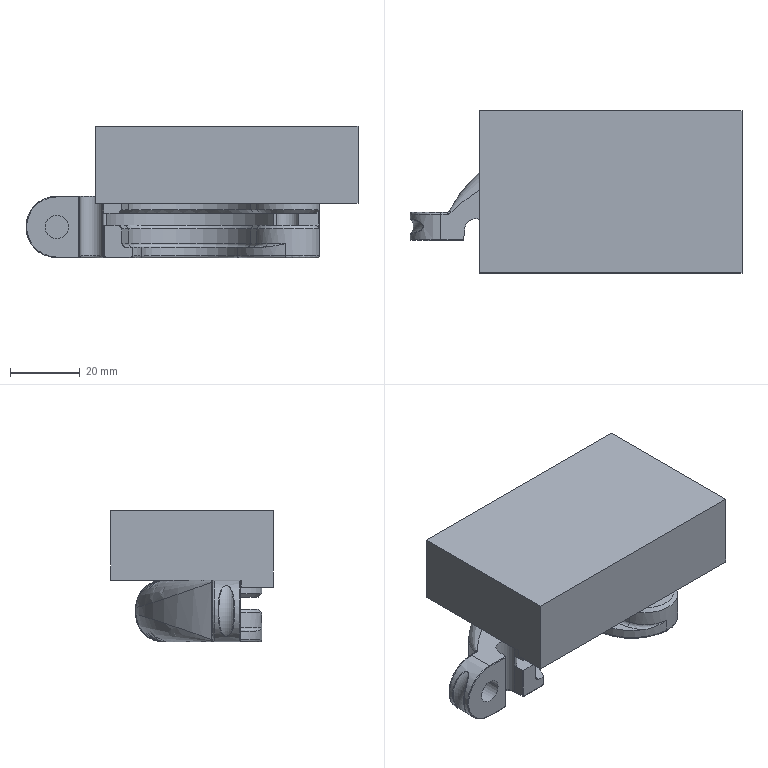NC program | NX | posted with a generic post | part box 94.951 x 46.35 x 37.6 mm
Lines 2348 to 3769 of 15115:
(PLANAR_MILL_3 , TOOL : D16)
N4592 T19 M6
N4594 G54
N4596 G17 G0 G90 X9.895 Y92.003 S5500 M3
N4598 G43 Z50. H19
N4600 Z16.9
N4602 G94 G1 X9.9 Y66.003 F2500.
N4604 Y64.053
N4606 G2 X9.855 Y62.913 R14.4
N4608 X5.16 Y52.857 R15.844
N4610 G3 X2.727 Y50.028 R35.618
N4612 X0.485 Y46.758 R34.794
N4614 X-2.476 Y40.54 R34.63
N4616 X-4.192 Y33.77 R36.295
N4618 X-4.497 Y30.926 R31.475
N4620 X-4.59 Y27.683 R50.37
N4622 X-4.539 Y22.92 R321.072
N4624 X-4.335 Y18.88 R62.671
N4626 X-3.595 Y14.096 R34.207
N4628 X-2.365 Y10.517 R17.742
N4630 X0.004 Y6.991 R13.901
N4632 X2.448 Y5.203 R7.84
N4634 G1 X26.001 Y-5.808
N4636 G0 Z22.4
N4638 X1.495 Y92.001
N4640 Z16.9
N4642 G1 X1.5 Y66.001
N4644 Y64.051
N4646 G2 X1.482 Y63.576 R6.
N4648 X-0.798 Y58.78 R7.444
N4650 G3 X-3.92 Y55.165 R44.018
N4652 X-6.702 Y51.105 R43.194
N4654 X-10.381 Y43.378 R43.03
N4656 X-12.496 Y35.042 R44.695
N4658 X-12.881 Y31.438 R39.875
N4660 X-12.99 Y27.655 R58.77
N4662 X-12.938 Y22.767 R329.472
N4664 X-12.707 Y18.186 R71.071
N4666 X-11.785 Y12.228 R42.607
N4668 X-9.971 Y6.954 R26.142
N4670 X-6.171 Y1.296 R22.301
N4672 X-1.11 Y-2.406 R16.24
N4674 G1 X22.443 Y-13.418
N4676 G0 Z22.4
N4678 X9.895 Y92.003
N4680 Z16.4
N4682 G1 X9.9 Y66.003
N4684 Y64.053
N4686 G2 X9.855 Y62.913 R14.4
N4688 X5.16 Y52.857 R15.844
N4690 G3 X2.727 Y50.028 R35.618
N4692 X0.485 Y46.758 R34.794
N4694 X-2.476 Y40.54 R34.63
N4696 X-4.192 Y33.77 R36.295
N4698 X-4.497 Y30.926 R31.475
N4700 X-4.59 Y27.683 R50.37
N4702 X-4.539 Y22.92 R321.072
N4704 X-4.335 Y18.88 R62.671
N4706 X-3.595 Y14.096 R34.207
N4708 X-2.365 Y10.517 R17.742
N4710 X0.004 Y6.991 R13.901
N4712 X2.448 Y5.203 R7.84
N4714 G1 X26.001 Y-5.808
N4716 G0 Z22.4
N4718 X1.495 Y92.001
N4720 Z16.4
N4722 G1 X1.5 Y66.001
N4724 Y64.051
N4726 G2 X1.482 Y63.576 R6.
N4728 X-0.798 Y58.78 R7.444
N4730 G3 X-3.92 Y55.165 R44.018
N4732 X-6.702 Y51.105 R43.194
N4734 X-10.381 Y43.378 R43.03
N4736 X-12.496 Y35.042 R44.695
N4738 X-12.881 Y31.438 R39.875
N4740 X-12.99 Y27.655 R58.77
N4742 X-12.938 Y22.767 R329.472
N4744 X-12.707 Y18.186 R71.071
N4746 X-11.785 Y12.228 R42.607
N4748 X-9.971 Y6.954 R26.142
N4750 X-6.171 Y1.296 R22.301
N4752 X-1.11 Y-2.406 R16.24
N4754 G1 X22.443 Y-13.418
N4756 G0 Z22.4
N4758 X9.895 Y92.003
N4760 Z15.9
N4762 G1 X9.9 Y66.003
N4764 Y64.053
N4766 G2 X9.855 Y62.913 R14.4
N4768 X5.16 Y52.857 R15.844
N4770 G3 X2.727 Y50.028 R35.618
N4772 X0.485 Y46.758 R34.794
N4774 X-2.476 Y40.54 R34.63
N4776 X-4.192 Y33.77 R36.295
N4778 X-4.497 Y30.926 R31.475
N4780 X-4.59 Y27.683 R50.37
N4782 X-4.539 Y22.92 R321.072
N4784 X-4.335 Y18.88 R62.671
N4786 X-3.595 Y14.096 R34.207
N4788 X-2.365 Y10.517 R17.742
N4790 X0.004 Y6.991 R13.901
N4792 X2.448 Y5.203 R7.84
N4794 G1 X26.001 Y-5.808
N4796 G0 Z22.4
N4798 X1.495 Y92.001
N4800 Z15.9
N4802 G1 X1.5 Y66.001
N4804 Y64.051
N4806 G2 X1.482 Y63.576 R6.
N4808 X-0.798 Y58.78 R7.444
N4810 G3 X-3.92 Y55.165 R44.018
N4812 X-6.702 Y51.105 R43.194
N4814 X-10.381 Y43.378 R43.03
N4816 X-12.496 Y35.042 R44.695
N4818 X-12.881 Y31.438 R39.875
N4820 X-12.99 Y27.655 R58.77
N4822 X-12.938 Y22.767 R329.472
N4824 X-12.707 Y18.186 R71.071
N4826 X-11.785 Y12.228 R42.607
N4828 X-9.971 Y6.954 R26.142
N4830 X-6.171 Y1.296 R22.301
N4832 X-1.11 Y-2.406 R16.24
N4834 G1 X22.443 Y-13.418
N4836 G0 Z22.4
N4838 X9.895 Y92.003
N4840 Z15.4
N4842 G1 X9.9 Y66.003
N4844 Y64.053
N4846 G2 X9.855 Y62.913 R14.4
N4848 X5.16 Y52.857 R15.844
N4850 G3 X2.727 Y50.028 R35.618
N4852 X0.485 Y46.758 R34.794
N4854 X-2.476 Y40.54 R34.63
N4856 X-4.192 Y33.77 R36.295
N4858 X-4.497 Y30.926 R31.475
N4860 X-4.59 Y27.683 R50.37
N4862 X-4.539 Y22.92 R321.072
N4864 X-4.335 Y18.88 R62.671
N4866 X-3.595 Y14.096 R34.207
N4868 X-2.365 Y10.517 R17.742
N4870 X0.004 Y6.991 R13.901
N4872 X2.448 Y5.203 R7.84
N4874 G1 X26.001 Y-5.808
N4876 G0 Z22.4
N4878 X1.495 Y92.001
N4880 Z15.4
N4882 G1 X1.5 Y66.001
N4884 Y64.051
N4886 G2 X1.482 Y63.576 R6.
N4888 X-0.798 Y58.78 R7.444
N4890 G3 X-3.92 Y55.165 R44.018
N4892 X-6.702 Y51.105 R43.194
N4894 X-10.381 Y43.378 R43.03
N4896 X-12.496 Y35.042 R44.695
N4898 X-12.881 Y31.438 R39.875
N4900 X-12.99 Y27.655 R58.77
N4902 X-12.938 Y22.767 R329.472
N4904 X-12.707 Y18.186 R71.071
N4906 X-11.785 Y12.228 R42.607
N4908 X-9.971 Y6.954 R26.142
N4910 X-6.171 Y1.296 R22.301
N4912 X-1.11 Y-2.406 R16.24
N4914 G1 X22.443 Y-13.418
N4916 G0 Z22.4
N4918 X9.895 Y92.003
N4920 Z14.9
N4922 G1 X9.9 Y66.003
N4924 Y64.053
N4926 G2 X9.855 Y62.913 R14.4
N4928 X5.16 Y52.857 R15.844
N4930 G3 X2.727 Y50.028 R35.618
N4932 X0.485 Y46.758 R34.794
N4934 X-2.476 Y40.54 R34.63
N4936 X-4.192 Y33.77 R36.295
N4938 X-4.497 Y30.926 R31.475
N4940 X-4.59 Y27.683 R50.37
N4942 X-4.539 Y22.92 R321.072
N4944 X-4.335 Y18.88 R62.671
N4946 X-3.595 Y14.096 R34.207
N4948 X-2.365 Y10.517 R17.742
N4950 X0.004 Y6.991 R13.901
N4952 X2.448 Y5.203 R7.84
N4954 G1 X26.001 Y-5.808
N4956 G0 Z22.4
N4958 X1.495 Y92.001
N4960 Z14.9
N4962 G1 X1.5 Y66.001
N4964 Y64.051
N4966 G2 X1.482 Y63.576 R6.
N4968 X-0.798 Y58.78 R7.444
N4970 G3 X-3.92 Y55.165 R44.018
N4972 X-6.702 Y51.105 R43.194
N4974 X-10.381 Y43.378 R43.03
N4976 X-12.496 Y35.042 R44.695
N4978 X-12.881 Y31.438 R39.875
N4980 X-12.99 Y27.655 R58.77
N4982 X-12.938 Y22.767 R329.472
N4984 X-12.707 Y18.186 R71.071
N4986 X-11.785 Y12.228 R42.607
N4988 X-9.971 Y6.954 R26.142
N4990 X-6.171 Y1.296 R22.301
N4992 X-1.11 Y-2.406 R16.24
N4994 G1 X22.443 Y-13.418
N4996 G0 Z22.4
N4998 X9.895 Y92.003
N5000 Z14.4
N5002 G1 X9.9 Y66.003
N5004 Y64.053
N5006 G2 X9.855 Y62.913 R14.4
N5008 X5.16 Y52.857 R15.844
N5010 G3 X2.727 Y50.028 R35.618
N5012 X0.485 Y46.758 R34.794
N5014 X-2.476 Y40.54 R34.63
N5016 X-4.192 Y33.77 R36.295
N5018 X-4.497 Y30.926 R31.475
N5020 X-4.59 Y27.683 R50.37
N5022 X-4.539 Y22.92 R321.072
N5024 X-4.335 Y18.88 R62.671
N5026 X-3.595 Y14.096 R34.207
N5028 X-2.365 Y10.517 R17.742
N5030 X0.004 Y6.991 R13.901
N5032 X2.448 Y5.203 R7.84
N5034 G1 X26.001 Y-5.808
N5036 G0 Z22.4
N5038 X1.495 Y92.001
N5040 Z14.4
N5042 G1 X1.5 Y66.001
N5044 Y64.051
N5046 G2 X1.482 Y63.576 R6.
N5048 X-0.798 Y58.78 R7.444
N5050 G3 X-3.92 Y55.165 R44.018
N5052 X-6.702 Y51.105 R43.194
N5054 X-10.381 Y43.378 R43.03
N5056 X-12.496 Y35.042 R44.695
N5058 X-12.881 Y31.438 R39.875
N5060 X-12.99 Y27.655 R58.77
N5062 X-12.938 Y22.767 R329.472
N5064 X-12.707 Y18.186 R71.071
N5066 X-11.785 Y12.228 R42.607
N5068 X-9.971 Y6.954 R26.142
N5070 X-6.171 Y1.296 R22.301
N5072 X-1.11 Y-2.406 R16.24
N5074 G1 X22.443 Y-13.418
N5076 G0 Z22.4
N5078 X9.895 Y92.003
N5080 Z13.9
N5082 G1 X9.9 Y66.003
N5084 Y64.053
N5086 G2 X9.855 Y62.913 R14.4
N5088 X5.16 Y52.857 R15.844
N5090 G3 X2.727 Y50.028 R35.618
N5092 X0.485 Y46.758 R34.794
N5094 X-2.476 Y40.54 R34.63
N5096 X-4.192 Y33.77 R36.295
N5098 X-4.497 Y30.926 R31.475
N5100 X-4.59 Y27.683 R50.37
N5102 X-4.539 Y22.92 R321.072
N5104 X-4.335 Y18.88 R62.671
N5106 X-3.595 Y14.096 R34.207
N5108 X-2.365 Y10.517 R17.742
N5110 X0.004 Y6.991 R13.901
N5112 X2.448 Y5.203 R7.84
N5114 G1 X26.001 Y-5.808
N5116 G0 Z22.4
N5118 X1.495 Y92.001
N5120 Z13.9
N5122 G1 X1.5 Y66.001
N5124 Y64.051
N5126 G2 X1.482 Y63.576 R6.
N5128 X-0.798 Y58.78 R7.444
N5130 G3 X-3.92 Y55.165 R44.018
N5132 X-6.702 Y51.105 R43.194
N5134 X-10.381 Y43.378 R43.03
N5136 X-12.496 Y35.042 R44.695
N5138 X-12.881 Y31.438 R39.875
N5140 X-12.99 Y27.655 R58.77
N5142 X-12.938 Y22.767 R329.472
N5144 X-12.707 Y18.186 R71.071
N5146 X-11.785 Y12.228 R42.607
N5148 X-9.971 Y6.954 R26.142
N5150 X-6.171 Y1.296 R22.301
N5152 X-1.11 Y-2.406 R16.24
N5154 G1 X22.443 Y-13.418
N5156 G0 Z22.4
N5158 X9.895 Y92.003
N5160 Z13.4
N5162 G1 X9.9 Y66.003
N5164 Y64.053
N5166 G2 X9.855 Y62.913 R14.4
N5168 X5.16 Y52.857 R15.844
N5170 G3 X2.727 Y50.028 R35.618
N5172 X0.485 Y46.758 R34.794
N5174 X-2.476 Y40.54 R34.63
N5176 X-4.192 Y33.77 R36.295
N5178 X-4.497 Y30.926 R31.475
N5180 X-4.59 Y27.683 R50.37
N5182 X-4.539 Y22.92 R321.072
N5184 X-4.335 Y18.88 R62.671
N5186 X-3.595 Y14.096 R34.207
N5188 X-2.365 Y10.517 R17.742
N5190 X0.004 Y6.991 R13.901
N5192 X2.448 Y5.203 R7.84
N5194 G1 X26.001 Y-5.808
N5196 G0 Z22.4
N5198 X1.495 Y92.001
N5200 Z13.4
N5202 G1 X1.5 Y66.001
N5204 Y64.051
N5206 G2 X1.482 Y63.576 R6.
N5208 X-0.798 Y58.78 R7.444
N5210 G3 X-3.92 Y55.165 R44.018
N5212 X-6.702 Y51.105 R43.194
N5214 X-10.381 Y43.378 R43.03
N5216 X-12.496 Y35.042 R44.695
N5218 X-12.881 Y31.438 R39.875
N5220 X-12.99 Y27.655 R58.77
N5222 X-12.938 Y22.767 R329.472
N5224 X-12.707 Y18.186 R71.071
N5226 X-11.785 Y12.228 R42.607
N5228 X-9.971 Y6.954 R26.142
N5230 X-6.171 Y1.296 R22.301
N5232 X-1.11 Y-2.406 R16.24
N5234 G1 X22.443 Y-13.418
N5236 G0 Z22.4
N5238 X9.895 Y92.003
N5240 Z12.9
N5242 G1 X9.9 Y66.003
N5244 Y64.053
N5246 G2 X9.855 Y62.913 R14.4
N5248 X5.16 Y52.857 R15.844
N5250 G3 X2.727 Y50.028 R35.618
N5252 X0.485 Y46.758 R34.794
N5254 X-2.476 Y40.54 R34.63
N5256 X-4.192 Y33.77 R36.295
N5258 X-4.497 Y30.926 R31.475
N5260 X-4.59 Y27.683 R50.37
N5262 X-4.539 Y22.92 R321.072
N5264 X-4.335 Y18.88 R62.671
N5266 X-3.595 Y14.096 R34.207
N5268 X-2.365 Y10.517 R17.742
N5270 X0.004 Y6.991 R13.901
N5272 X2.448 Y5.203 R7.84
N5274 G1 X26.001 Y-5.808
N5276 G0 Z22.4
N5278 X1.495 Y92.001
N5280 Z12.9
N5282 G1 X1.5 Y66.001
N5284 Y64.051
N5286 G2 X1.482 Y63.576 R6.
N5288 X-0.798 Y58.78 R7.444
N5290 G3 X-3.92 Y55.165 R44.018
N5292 X-6.702 Y51.105 R43.194
N5294 X-10.381 Y43.378 R43.03
N5296 X-12.496 Y35.042 R44.695
N5298 X-12.881 Y31.438 R39.875
N5300 X-12.99 Y27.655 R58.77
N5302 X-12.938 Y22.767 R329.472
N5304 X-12.707 Y18.186 R71.071
N5306 X-11.785 Y12.228 R42.607
N5308 X-9.971 Y6.954 R26.142
N5310 X-6.171 Y1.296 R22.301
N5312 X-1.11 Y-2.406 R16.24
N5314 G1 X22.443 Y-13.418
N5316 G0 Z22.4
N5318 X9.895 Y92.003
N5320 Z12.4
N5322 G1 X9.9 Y66.003
N5324 Y64.053
N5326 G2 X9.855 Y62.913 R14.4
N5328 X5.16 Y52.857 R15.844
N5330 G3 X2.727 Y50.028 R35.618
N5332 X0.485 Y46.758 R34.794
N5334 X-2.476 Y40.54 R34.63
N5336 X-4.192 Y33.77 R36.295
N5338 X-4.497 Y30.926 R31.475
N5340 X-4.59 Y27.683 R50.37
N5342 X-4.539 Y22.92 R321.072
N5344 X-4.335 Y18.88 R62.671
N5346 X-3.595 Y14.096 R34.207
N5348 X-2.365 Y10.517 R17.742
N5350 X0.004 Y6.991 R13.901
N5352 X2.448 Y5.203 R7.84
N5354 G1 X26.001 Y-5.808
N5356 G0 Z22.4
N5358 X1.495 Y92.001
N5360 Z12.4
N5362 G1 X1.5 Y66.001
N5364 Y64.051
N5366 G2 X1.482 Y63.576 R6.
N5368 X-0.798 Y58.78 R7.444
N5370 G3 X-3.92 Y55.165 R44.018
N5372 X-6.702 Y51.105 R43.194
N5374 X-10.381 Y43.378 R43.03
N5376 X-12.496 Y35.042 R44.695
N5378 X-12.881 Y31.438 R39.875
N5380 X-12.99 Y27.655 R58.77
N5382 X-12.938 Y22.767 R329.472
N5384 X-12.707 Y18.186 R71.071
N5386 X-11.785 Y12.228 R42.607
N5388 X-9.971 Y6.954 R26.142
N5390 X-6.171 Y1.296 R22.301
N5392 X-1.11 Y-2.406 R16.24
N5394 G1 X22.443 Y-13.418
N5396 G0 Z22.4
N5398 X9.895 Y92.003
N5400 Z11.9
N5402 G1 X9.9 Y66.003
N5404 Y64.053
N5406 G2 X9.855 Y62.913 R14.4
N5408 X5.16 Y52.857 R15.844
N5410 G3 X2.727 Y50.028 R35.618
N5412 X0.485 Y46.758 R34.794
N5414 X-2.476 Y40.54 R34.63
N5416 X-4.192 Y33.77 R36.295
N5418 X-4.497 Y30.926 R31.475
N5420 X-4.59 Y27.683 R50.37
N5422 X-4.539 Y22.92 R321.072
N5424 X-4.335 Y18.88 R62.671
N5426 X-3.595 Y14.096 R34.207
N5428 X-2.365 Y10.517 R17.742
N5430 X0.004 Y6.991 R13.901
N5432 X2.448 Y5.203 R7.84
N5434 G1 X26.001 Y-5.808
N5436 G0 Z22.4
N5438 X1.495 Y92.001
N5440 Z11.9
N5442 G1 X1.5 Y66.001
N5444 Y64.051
N5446 G2 X1.482 Y63.576 R6.
N5448 X-0.798 Y58.78 R7.444
N5450 G3 X-3.92 Y55.165 R44.018
N5452 X-6.702 Y51.105 R43.194
N5454 X-10.381 Y43.378 R43.03
N5456 X-12.496 Y35.042 R44.695
N5458 X-12.881 Y31.438 R39.875
N5460 X-12.99 Y27.655 R58.77
N5462 X-12.938 Y22.767 R329.472
N5464 X-12.707 Y18.186 R71.071
N5466 X-11.785 Y12.228 R42.607
N5468 X-9.971 Y6.954 R26.142
N5470 X-6.171 Y1.296 R22.301
N5472 X-1.11 Y-2.406 R16.24
N5474 G1 X22.443 Y-13.418
N5476 G0 Z22.4
N5478 X9.895 Y92.003
N5480 Z11.4
N5482 G1 X9.9 Y66.003
N5484 Y64.053
N5486 G2 X9.855 Y62.913 R14.4
N5488 X5.16 Y52.857 R15.844
N5490 G3 X2.727 Y50.028 R35.618
N5492 X0.485 Y46.758 R34.794
N5494 X-2.476 Y40.54 R34.63
N5496 X-4.192 Y33.77 R36.295
N5498 X-4.497 Y30.926 R31.475
N5500 X-4.59 Y27.683 R50.37
N5502 X-4.539 Y22.92 R321.072
N5504 X-4.335 Y18.88 R62.671
N5506 X-3.595 Y14.096 R34.207
N5508 X-2.365 Y10.517 R17.742
N5510 X0.004 Y6.991 R13.901
N5512 X2.448 Y5.203 R7.84
N5514 G1 X26.001 Y-5.808
N5516 G0 Z22.4
N5518 X1.495 Y92.001
N5520 Z11.4
N5522 G1 X1.5 Y66.001
N5524 Y64.051
N5526 G2 X1.482 Y63.576 R6.
N5528 X-0.798 Y58.78 R7.444
N5530 G3 X-3.92 Y55.165 R44.018
N5532 X-6.702 Y51.105 R43.194
N5534 X-10.381 Y43.378 R43.03
N5536 X-12.496 Y35.042 R44.695
N5538 X-12.881 Y31.438 R39.875
N5540 X-12.99 Y27.655 R58.77
N5542 X-12.938 Y22.767 R329.472
N5544 X-12.707 Y18.186 R71.071
N5546 X-11.785 Y12.228 R42.607
N5548 X-9.971 Y6.954 R26.142
N5550 X-6.171 Y1.296 R22.301
N5552 X-1.11 Y-2.406 R16.24
N5554 G1 X22.443 Y-13.418
N5556 G0 Z22.4
N5558 X9.895 Y92.003
N5560 Z10.9
N5562 G1 X9.9 Y66.003
N5564 Y64.053
N5566 G2 X9.855 Y62.913 R14.4
N5568 X5.16 Y52.857 R15.844
N5570 G3 X2.727 Y50.028 R35.618
N5572 X0.485 Y46.758 R34.794
N5574 X-2.476 Y40.54 R34.63
N5576 X-4.192 Y33.77 R36.295
N5578 X-4.497 Y30.926 R31.475
N5580 X-4.59 Y27.683 R50.37
N5582 X-4.539 Y22.92 R321.072
N5584 X-4.335 Y18.88 R62.671
N5586 X-3.595 Y14.096 R34.207
N5588 X-2.365 Y10.517 R17.742
N5590 X0.004 Y6.991 R13.901
N5592 X2.448 Y5.203 R7.84
N5594 G1 X26.001 Y-5.808
N5596 G0 Z22.4
N5598 X1.495 Y92.001
N5600 Z10.9
N5602 G1 X1.5 Y66.001
N5604 Y64.051
N5606 G2 X1.482 Y63.576 R6.
N5608 X-0.798 Y58.78 R7.444
N5610 G3 X-3.92 Y55.165 R44.018
N5612 X-6.702 Y51.105 R43.194
N5614 X-10.381 Y43.378 R43.03
N5616 X-12.496 Y35.042 R44.695
N5618 X-12.881 Y31.438 R39.875
N5620 X-12.99 Y27.655 R58.77
N5622 X-12.938 Y22.767 R329.472
N5624 X-12.707 Y18.186 R71.071
N5626 X-11.785 Y12.228 R42.607
N5628 X-9.971 Y6.954 R26.142
N5630 X-6.171 Y1.296 R22.301
N5632 X-1.11 Y-2.406 R16.24
N5634 G1 X22.443 Y-13.418
N5636 G0 Z22.4
N5638 X9.895 Y92.003
N5640 Z10.4
N5642 G1 X9.9 Y66.003
N5644 Y64.053
N5646 G2 X9.855 Y62.913 R14.4
N5648 X5.16 Y52.857 R15.844
N5650 G3 X2.727 Y50.028 R35.618
N5652 X0.485 Y46.758 R34.794
N5654 X-2.476 Y40.54 R34.63
N5656 X-4.192 Y33.77 R36.295
N5658 X-4.497 Y30.926 R31.475
N5660 X-4.59 Y27.683 R50.37
N5662 X-4.539 Y22.92 R321.072
N5664 X-4.335 Y18.88 R62.671
N5666 X-3.595 Y14.096 R34.207
N5668 X-2.365 Y10.517 R17.742
N5670 X0.004 Y6.991 R13.901
N5672 X2.448 Y5.203 R7.84
N5674 G1 X26.001 Y-5.808
N5676 G0 Z22.4
N5678 X1.495 Y92.001
N5680 Z10.4
N5682 G1 X1.5 Y66.001
N5684 Y64.051
N5686 G2 X1.482 Y63.576 R6.
N5688 X-0.798 Y58.78 R7.444
N5690 G3 X-3.92 Y55.165 R44.018
N5692 X-6.702 Y51.105 R43.194
N5694 X-10.381 Y43.378 R43.03
N5696 X-12.496 Y35.042 R44.695
N5698 X-12.881 Y31.438 R39.875
N5700 X-12.99 Y27.655 R58.77
N5702 X-12.938 Y22.767 R329.472
N5704 X-12.707 Y18.186 R71.071
N5706 X-11.785 Y12.228 R42.607
N5708 X-9.971 Y6.954 R26.142
N5710 X-6.171 Y1.296 R22.301
N5712 X-1.11 Y-2.406 R16.24
N5714 G1 X22.443 Y-13.418
N5716 G0 Z22.4
N5718 X9.895 Y92.003
N5720 Z9.9
N5722 G1 X9.9 Y66.003
N5724 Y64.053
N5726 G2 X9.855 Y62.913 R14.4
N5728 X5.16 Y52.857 R15.844
N5730 G3 X2.727 Y50.028 R35.618
N5732 X0.485 Y46.758 R34.794
N5734 X-2.476 Y40.54 R34.63
N5736 X-4.192 Y33.77 R36.295
N5738 X-4.497 Y30.926 R31.475
N5740 X-4.59 Y27.683 R50.37
N5742 X-4.539 Y22.92 R321.072
N5744 X-4.335 Y18.88 R62.671
N5746 X-3.595 Y14.096 R34.207
N5748 X-2.365 Y10.517 R17.742
N5750 X0.004 Y6.991 R13.901
N5752 X2.448 Y5.203 R7.84
N5754 G1 X26.001 Y-5.808
N5756 G0 Z22.4
N5758 X1.495 Y92.001
N5760 Z9.9
N5762 G1 X1.5 Y66.001
N5764 Y64.051
N5766 G2 X1.482 Y63.576 R6.
N5768 X-0.798 Y58.78 R7.444
N5770 G3 X-3.92 Y55.165 R44.018
N5772 X-6.702 Y51.105 R43.194
N5774 X-10.381 Y43.378 R43.03
N5776 X-12.496 Y35.042 R44.695
N5778 X-12.881 Y31.438 R39.875
N5780 X-12.99 Y27.655 R58.77
N5782 X-12.938 Y22.767 R329.472
N5784 X-12.707 Y18.186 R71.071
N5786 X-11.785 Y12.228 R42.607
N5788 X-9.971 Y6.954 R26.142
N5790 X-6.171 Y1.296 R22.301
N5792 X-1.11 Y-2.406 R16.24
N5794 G1 X22.443 Y-13.418
N5796 G0 Z22.4
N5798 X9.895 Y92.003
N5800 Z9.4
N5802 G1 X9.9 Y66.003
N5804 Y64.053
N5806 G2 X9.855 Y62.913 R14.4
N5808 X5.16 Y52.857 R15.844
N5810 G3 X2.727 Y50.028 R35.618
N5812 X0.485 Y46.758 R34.794
N5814 X-2.476 Y40.54 R34.63
N5816 X-4.192 Y33.77 R36.295
N5818 X-4.497 Y30.926 R31.475
N5820 X-4.59 Y27.683 R50.37
N5822 X-4.539 Y22.92 R321.072
N5824 X-4.335 Y18.88 R62.671
N5826 X-3.595 Y14.096 R34.207
N5828 X-2.365 Y10.517 R17.742
N5830 X0.004 Y6.991 R13.901
N5832 X2.448 Y5.203 R7.84
N5834 G1 X26.001 Y-5.808
N5836 G0 Z22.4
N5838 X1.495 Y92.001
N5840 Z9.4
N5842 G1 X1.5 Y66.001
N5844 Y64.051
N5846 G2 X1.482 Y63.576 R6.
N5848 X-0.798 Y58.78 R7.444
N5850 G3 X-3.92 Y55.165 R44.018
N5852 X-6.702 Y51.105 R43.194
N5854 X-10.381 Y43.378 R43.03
N5856 X-12.496 Y35.042 R44.695
N5858 X-12.881 Y31.438 R39.875
N5860 X-12.99 Y27.655 R58.77
N5862 X-12.938 Y22.767 R329.472
N5864 X-12.707 Y18.186 R71.071
N5866 X-11.785 Y12.228 R42.607
N5868 X-9.971 Y6.954 R26.142
N5870 X-6.171 Y1.296 R22.301
N5872 X-1.11 Y-2.406 R16.24
N5874 G1 X22.443 Y-13.418
N5876 G0 Z22.4
N5878 X9.895 Y92.003
N5880 Z8.9
N5882 G1 X9.9 Y66.003
N5884 Y64.053
N5886 G2 X9.855 Y62.913 R14.4
N5888 X5.16 Y52.857 R15.844
N5890 G3 X2.727 Y50.028 R35.618
N5892 X0.485 Y46.758 R34.794
N5894 X-2.476 Y40.54 R34.63
N5896 X-4.192 Y33.77 R36.295
N5898 X-4.497 Y30.926 R31.475
N5900 X-4.59 Y27.683 R50.37
N5902 X-4.539 Y22.92 R321.072
N5904 X-4.335 Y18.88 R62.671
N5906 X-3.595 Y14.096 R34.207
N5908 X-2.365 Y10.517 R17.742
N5910 X0.004 Y6.991 R13.901
N5912 X2.448 Y5.203 R7.84
N5914 G1 X26.001 Y-5.808
N5916 G0 Z22.4
N5918 X1.495 Y92.001
N5920 Z8.9
N5922 G1 X1.5 Y66.001
N5924 Y64.051
N5926 G2 X1.482 Y63.576 R6.
N5928 X-0.798 Y58.78 R7.444
N5930 G3 X-3.92 Y55.165 R44.018
N5932 X-6.702 Y51.105 R43.194
N5934 X-10.381 Y43.378 R43.03
N5936 X-12.496 Y35.042 R44.695
N5938 X-12.881 Y31.438 R39.875
N5940 X-12.99 Y27.655 R58.77
N5942 X-12.938 Y22.767 R329.472
N5944 X-12.707 Y18.186 R71.071
N5946 X-11.785 Y12.228 R42.607
N5948 X-9.971 Y6.954 R26.142
N5950 X-6.171 Y1.296 R22.301
N5952 X-1.11 Y-2.406 R16.24
N5954 G1 X22.443 Y-13.418
N5956 G0 Z22.4
N5958 X9.895 Y92.003
N5960 Z8.4
N5962 G1 X9.9 Y66.003
N5964 Y64.053
N5966 G2 X9.855 Y62.913 R14.4
N5968 X5.16 Y52.857 R15.844
N5970 G3 X2.727 Y50.028 R35.618
N5972 X0.485 Y46.758 R34.794
N5974 X-2.476 Y40.54 R34.63
N5976 X-4.192 Y33.77 R36.295
N5978 X-4.497 Y30.926 R31.475
N5980 X-4.59 Y27.683 R50.37
N5982 X-4.539 Y22.92 R321.072
N5984 X-4.335 Y18.88 R62.671
N5986 X-3.595 Y14.096 R34.207
N5988 X-2.365 Y10.517 R17.742
N5990 X0.004 Y6.991 R13.901
N5992 X2.448 Y5.203 R7.84
N5994 G1 X26.001 Y-5.808
N5996 G0 Z22.4
N5998 X1.495 Y92.001
N6000 Z8.4
N6002 G1 X1.5 Y66.001
N6004 Y64.051
N6006 G2 X1.482 Y63.576 R6.
N6008 X-0.798 Y58.78 R7.444
N6010 G3 X-3.92 Y55.165 R44.018
N6012 X-6.702 Y51.105 R43.194
N6014 X-10.381 Y43.378 R43.03
N6016 X-12.496 Y35.042 R44.695
N6018 X-12.881 Y31.438 R39.875
N6020 X-12.99 Y27.655 R58.77
N6022 X-12.938 Y22.767 R329.472
N6024 X-12.707 Y18.186 R71.071
N6026 X-11.785 Y12.228 R42.607
N6028 X-9.971 Y6.954 R26.142
N6030 X-6.171 Y1.296 R22.301
N6032 X-1.11 Y-2.406 R16.24
N6034 G1 X22.443 Y-13.418
N6036 G0 Z22.4
N6038 X9.895 Y92.003
N6040 Z7.9
N6042 G1 X9.9 Y66.003
N6044 Y64.053
N6046 G2 X9.855 Y62.913 R14.4
N6048 X5.16 Y52.857 R15.844
N6050 G3 X2.727 Y50.028 R35.618
N6052 X0.485 Y46.758 R34.794
N6054 X-2.476 Y40.54 R34.63
N6056 X-4.192 Y33.77 R36.295
N6058 X-4.497 Y30.926 R31.475
N6060 X-4.59 Y27.683 R50.37
N6062 X-4.539 Y22.92 R321.072
N6064 X-4.335 Y18.88 R62.671
N6066 X-3.595 Y14.096 R34.207
N6068 X-2.365 Y10.517 R17.742
N6070 X0.004 Y6.991 R13.901
N6072 X2.448 Y5.203 R7.84
N6074 G1 X26.001 Y-5.808
N6076 G0 Z22.4
N6078 X1.495 Y92.001
N6080 Z7.9
N6082 G1 X1.5 Y66.001
N6084 Y64.051
N6086 G2 X1.482 Y63.576 R6.
N6088 X-0.798 Y58.78 R7.444
N6090 G3 X-3.92 Y55.165 R44.018
N6092 X-6.702 Y51.105 R43.194
N6094 X-10.381 Y43.378 R43.03
N6096 X-12.496 Y35.042 R44.695
N6098 X-12.881 Y31.438 R39.875
N6100 X-12.99 Y27.655 R58.77
N6102 X-12.938 Y22.767 R329.472
N6104 X-12.707 Y18.186 R71.071
N6106 X-11.785 Y12.228 R42.607
N6108 X-9.971 Y6.954 R26.142
N6110 X-6.171 Y1.296 R22.301
N6112 X-1.11 Y-2.406 R16.24
N6114 G1 X22.443 Y-13.418
N6116 G0 Z22.4
N6118 X9.895 Y92.003
N6120 Z7.4
N6122 G1 X9.9 Y66.003
N6124 Y64.053
N6126 G2 X9.855 Y62.913 R14.4
N6128 X5.16 Y52.857 R15.844
N6130 G3 X2.727 Y50.028 R35.618
N6132 X0.485 Y46.758 R34.794
N6134 X-2.476 Y40.54 R34.63
N6136 X-4.192 Y33.77 R36.295
N6138 X-4.497 Y30.926 R31.475
N6140 X-4.59 Y27.683 R50.37
N6142 X-4.539 Y22.92 R321.072
N6144 X-4.335 Y18.88 R62.671
N6146 X-3.595 Y14.096 R34.207
N6148 X-2.365 Y10.517 R17.742
N6150 X0.004 Y6.991 R13.901
N6152 X2.448 Y5.203 R7.84
N6154 G1 X26.001 Y-5.808
N6156 G0 Z22.4
N6158 X1.495 Y92.001
N6160 Z7.4
N6162 G1 X1.5 Y66.001
N6164 Y64.051
N6166 G2 X1.482 Y63.576 R6.
N6168 X-0.798 Y58.78 R7.444
N6170 G3 X-3.92 Y55.165 R44.018
N6172 X-6.702 Y51.105 R43.194
N6174 X-10.381 Y43.378 R43.03
N6176 X-12.496 Y35.042 R44.695
N6178 X-12.881 Y31.438 R39.875
N6180 X-12.99 Y27.655 R58.77
N6182 X-12.938 Y22.767 R329.472
N6184 X-12.707 Y18.186 R71.071
N6186 X-11.785 Y12.228 R42.607
N6188 X-9.971 Y6.954 R26.142
N6190 X-6.171 Y1.296 R22.301
N6192 X-1.11 Y-2.406 R16.24
N6194 G1 X22.443 Y-13.418
N6196 G0 Z22.4
N6198 X9.895 Y92.003
N6200 Z6.9
N6202 G1 X9.9 Y66.003
N6204 Y64.053
N6206 G2 X9.855 Y62.913 R14.4
N6208 X5.16 Y52.857 R15.844
N6210 G3 X2.727 Y50.028 R35.618
N6212 X0.485 Y46.758 R34.794
N6214 X-2.476 Y40.54 R34.63
N6216 X-4.192 Y33.77 R36.295
N6218 X-4.497 Y30.926 R31.475
N6220 X-4.59 Y27.683 R50.37
N6222 X-4.539 Y22.92 R321.072
N6224 X-4.335 Y18.88 R62.671
N6226 X-3.595 Y14.096 R34.207
N6228 X-2.365 Y10.517 R17.742
N6230 X0.004 Y6.991 R13.901
N6232 X2.448 Y5.203 R7.84
N6234 G1 X26.001 Y-5.808
N6236 G0 Z22.4
N6238 X1.495 Y92.001
N6240 Z6.9
N6242 G1 X1.5 Y66.001
N6244 Y64.051
N6246 G2 X1.482 Y63.576 R6.
N6248 X-0.798 Y58.78 R7.444
N6250 G3 X-3.92 Y55.165 R44.018
N6252 X-6.702 Y51.105 R43.194
N6254 X-10.381 Y43.378 R43.03
N6256 X-12.496 Y35.042 R44.695
N6258 X-12.881 Y31.438 R39.875
N6260 X-12.99 Y27.655 R58.77
N6262 X-12.938 Y22.767 R329.472
N6264 X-12.707 Y18.186 R71.071
N6266 X-11.785 Y12.228 R42.607
N6268 X-9.971 Y6.954 R26.142
N6270 X-6.171 Y1.296 R22.301
N6272 X-1.11 Y-2.406 R16.24
N6274 G1 X22.443 Y-13.418
N6276 G0 Z22.4
N6278 X9.895 Y92.003
N6280 Z6.4
N6282 G1 X9.9 Y66.003
N6284 Y64.053
N6286 G2 X9.855 Y62.913 R14.4
N6288 X5.16 Y52.857 R15.844
N6290 G3 X2.727 Y50.028 R35.618
N6292 X0.485 Y46.758 R34.794
N6294 X-2.476 Y40.54 R34.63
N6296 X-4.192 Y33.77 R36.295
N6298 X-4.497 Y30.926 R31.475
N6300 X-4.59 Y27.683 R50.37
N6302 X-4.539 Y22.92 R321.072
N6304 X-4.335 Y18.88 R62.671
N6306 X-3.595 Y14.096 R34.207
N6308 X-2.365 Y10.517 R17.742
N6310 X0.004 Y6.991 R13.901
N6312 X2.448 Y5.203 R7.84
N6314 G1 X26.001 Y-5.808
N6316 G0 Z22.4
N6318 X1.495 Y92.001
N6320 Z6.4
N6322 G1 X1.5 Y66.001
N6324 Y64.051
N6326 G2 X1.482 Y63.576 R6.
N6328 X-0.798 Y58.78 R7.444
N6330 G3 X-3.92 Y55.165 R44.018
N6332 X-6.702 Y51.105 R43.194
N6334 X-10.381 Y43.378 R43.03
N6336 X-12.496 Y35.042 R44.695
N6338 X-12.881 Y31.438 R39.875
N6340 X-12.99 Y27.655 R58.77
N6342 X-12.938 Y22.767 R329.472
N6344 X-12.707 Y18.186 R71.071
N6346 X-11.785 Y12.228 R42.607
N6348 X-9.971 Y6.954 R26.142
N6350 X-6.171 Y1.296 R22.301
N6352 X-1.11 Y-2.406 R16.24
N6354 G1 X22.443 Y-13.418
N6356 G0 Z22.4
N6358 X9.895 Y92.003
N6360 Z5.9
N6362 G1 X9.9 Y66.003
N6364 Y64.053
N6366 G2 X9.855 Y62.913 R14.4
N6368 X5.16 Y52.857 R15.844
N6370 G3 X2.727 Y50.028 R35.618
N6372 X0.485 Y46.758 R34.794
N6374 X-2.476 Y40.54 R34.63
N6376 X-4.192 Y33.77 R36.295
N6378 X-4.497 Y30.926 R31.475
N6380 X-4.59 Y27.683 R50.37
N6382 X-4.539 Y22.92 R321.072
N6384 X-4.335 Y18.88 R62.671
N6386 X-3.595 Y14.096 R34.207
N6388 X-2.365 Y10.517 R17.742
N6390 X0.004 Y6.991 R13.901
N6392 X2.448 Y5.203 R7.84
N6394 G1 X26.001 Y-5.808
N6396 G0 Z22.4
N6398 X1.495 Y92.001
N6400 Z5.9
N6402 G1 X1.5 Y66.001
N6404 Y64.051
N6406 G2 X1.482 Y63.576 R6.
N6408 X-0.798 Y58.78 R7.444
N6410 G3 X-3.92 Y55.165 R44.018
N6412 X-6.702 Y51.105 R43.194
N6414 X-10.381 Y43.378 R43.03
N6416 X-12.496 Y35.042 R44.695
N6418 X-12.881 Y31.438 R39.875
N6420 X-12.99 Y27.655 R58.77
N6422 X-12.938 Y22.767 R329.472
N6424 X-12.707 Y18.186 R71.071
N6426 X-11.785 Y12.228 R42.607
N6428 X-9.971 Y6.954 R26.142
N6430 X-6.171 Y1.296 R22.301
N6432 X-1.11 Y-2.406 R16.24
N6434 G1 X22.443 Y-13.418
N6436 G0 Z22.4
N6438 X9.895 Y92.003
N6440 Z5.4
N6442 G1 X9.9 Y66.003
N6444 Y64.053
N6446 G2 X9.855 Y62.913 R14.4
N6448 X5.16 Y52.857 R15.844
N6450 G3 X2.727 Y50.028 R35.618
N6452 X0.485 Y46.758 R34.794
N6454 X-2.476 Y40.54 R34.63
N6456 X-4.192 Y33.77 R36.295
N6458 X-4.497 Y30.926 R31.475
N6460 X-4.59 Y27.683 R50.37
N6462 X-4.539 Y22.92 R321.072
N6464 X-4.335 Y18.88 R62.671
N6466 X-3.595 Y14.096 R34.207
N6468 X-2.365 Y10.517 R17.742
N6470 X0.004 Y6.991 R13.901
N6472 X2.448 Y5.203 R7.84
N6474 G1 X26.001 Y-5.808
N6476 G0 Z22.4
N6478 X1.495 Y92.001
N6480 Z5.4
N6482 G1 X1.5 Y66.001
N6484 Y64.051
N6486 G2 X1.482 Y63.576 R6.
N6488 X-0.798 Y58.78 R7.444
N6490 G3 X-3.92 Y55.165 R44.018
N6492 X-6.702 Y51.105 R43.194
N6494 X-10.381 Y43.378 R43.03
N6496 X-12.496 Y35.042 R44.695
N6498 X-12.881 Y31.438 R39.875
N6500 X-12.99 Y27.655 R58.77
N6502 X-12.938 Y22.767 R329.472
N6504 X-12.707 Y18.186 R71.071
N6506 X-11.785 Y12.228 R42.607
N6508 X-9.971 Y6.954 R26.142
N6510 X-6.171 Y1.296 R22.301
N6512 X-1.11 Y-2.406 R16.24
N6514 G1 X22.443 Y-13.418
N6516 G0 Z22.4
N6518 X9.895 Y92.003
N6520 Z4.9
N6522 G1 X9.9 Y66.003
N6524 Y64.053
N6526 G2 X9.855 Y62.913 R14.4
N6528 X5.16 Y52.857 R15.844
N6530 G3 X2.727 Y50.028 R35.618
N6532 X0.485 Y46.758 R34.794
N6534 X-2.476 Y40.54 R34.63
N6536 X-4.192 Y33.77 R36.295
N6538 X-4.497 Y30.926 R31.475
N6540 X-4.59 Y27.683 R50.37
N6542 X-4.539 Y22.92 R321.072
N6544 X-4.335 Y18.88 R62.671
N6546 X-3.595 Y14.096 R34.207
N6548 X-2.365 Y10.517 R17.742
N6550 X0.004 Y6.991 R13.901
N6552 X2.448 Y5.203 R7.84
N6554 G1 X26.001 Y-5.808
N6556 G0 Z22.4
N6558 X1.495 Y92.001
N6560 Z4.9
N6562 G1 X1.5 Y66.001
N6564 Y64.051
N6566 G2 X1.482 Y63.576 R6.
N6568 X-0.798 Y58.78 R7.444
N6570 G3 X-3.92 Y55.165 R44.018
N6572 X-6.702 Y51.105 R43.194
N6574 X-10.381 Y43.378 R43.03
N6576 X-12.496 Y35.042 R44.695
N6578 X-12.881 Y31.438 R39.875
N6580 X-12.99 Y27.655 R58.77
N6582 X-12.938 Y22.767 R329.472
N6584 X-12.707 Y18.186 R71.071
N6586 X-11.785 Y12.228 R42.607
N6588 X-9.971 Y6.954 R26.142
N6590 X-6.171 Y1.296 R22.301
N6592 X-1.11 Y-2.406 R16.24
N6594 G1 X22.443 Y-13.418
N6596 G0 Z22.4
N6598 X9.895 Y92.003
N6600 Z4.4
N6602 G1 X9.9 Y66.003
N6604 Y64.053
N6606 G2 X9.855 Y62.913 R14.4
N6608 X5.16 Y52.857 R15.844
N6610 G3 X2.727 Y50.028 R35.618
N6612 X0.485 Y46.758 R34.794
N6614 X-2.476 Y40.54 R34.63
N6616 X-4.192 Y33.77 R36.295
N6618 X-4.497 Y30.926 R31.475
N6620 X-4.59 Y27.683 R50.37
N6622 X-4.539 Y22.92 R321.072
N6624 X-4.335 Y18.88 R62.671
N6626 X-3.595 Y14.096 R34.207
N6628 X-2.365 Y10.517 R17.742
N6630 X0.004 Y6.991 R13.901
N6632 X2.448 Y5.203 R7.84
N6634 G1 X26.001 Y-5.808
N6636 G0 Z22.4
N6638 X1.495 Y92.001
N6640 Z4.4
N6642 G1 X1.5 Y66.001
N6644 Y64.051
N6646 G2 X1.482 Y63.576 R6.
N6648 X-0.798 Y58.78 R7.444
N6650 G3 X-3.92 Y55.165 R44.018
N6652 X-6.702 Y51.105 R43.194
N6654 X-10.381 Y43.378 R43.03
N6656 X-12.496 Y35.042 R44.695
N6658 X-12.881 Y31.438 R39.875
N6660 X-12.99 Y27.655 R58.77
N6662 X-12.938 Y22.767 R329.472
N6664 X-12.707 Y18.186 R71.071
N6666 X-11.785 Y12.228 R42.607
N6668 X-9.971 Y6.954 R26.142
N6670 X-6.171 Y1.296 R22.301
N6672 X-1.11 Y-2.406 R16.24
N6674 G1 X22.443 Y-13.418
N6676 G0 Z22.4
N6678 X9.895 Y92.003
N6680 Z3.9
N6682 G1 X9.9 Y66.003
N6684 Y64.053
N6686 G2 X9.855 Y62.913 R14.4
N6688 X5.16 Y52.857 R15.844
N6690 G3 X2.727 Y50.028 R35.618
N6692 X0.485 Y46.758 R34.794
N6694 X-2.476 Y40.54 R34.63
N6696 X-4.192 Y33.77 R36.295
N6698 X-4.497 Y30.926 R31.475
N6700 X-4.59 Y27.683 R50.37
N6702 X-4.539 Y22.92 R321.072
N6704 X-4.335 Y18.88 R62.671
N6706 X-3.595 Y14.096 R34.207
N6708 X-2.365 Y10.517 R17.742
N6710 X0.004 Y6.991 R13.901
N6712 X2.448 Y5.203 R7.84
N6714 G1 X26.001 Y-5.808
N6716 G0 Z22.4
N6718 X1.495 Y92.001
N6720 Z3.9
N6722 G1 X1.5 Y66.001
N6724 Y64.051
N6726 G2 X1.482 Y63.576 R6.
N6728 X-0.798 Y58.78 R7.444
N6730 G3 X-3.92 Y55.165 R44.018
N6732 X-6.702 Y51.105 R43.194
N6734 X-10.381 Y43.378 R43.03
N6736 X-12.496 Y35.042 R44.695
N6738 X-12.881 Y31.438 R39.875
N6740 X-12.99 Y27.655 R58.77
N6742 X-12.938 Y22.767 R329.472
N6744 X-12.707 Y18.186 R71.071
N6746 X-11.785 Y12.228 R42.607
N6748 X-9.971 Y6.954 R26.142
N6750 X-6.171 Y1.296 R22.301
N6752 X-1.11 Y-2.406 R16.24
N6754 G1 X22.443 Y-13.418
N6756 G0 Z22.4
N6758 X9.895 Y92.003
N6760 Z3.4
N6762 G1 X9.9 Y66.003
N6764 Y64.053
N6766 G2 X9.855 Y62.913 R14.4
N6768 X5.16 Y52.857 R15.844
N6770 G3 X2.727 Y50.028 R35.618
N6772 X0.485 Y46.758 R34.794
N6774 X-2.476 Y40.54 R34.63
N6776 X-4.192 Y33.77 R36.295
N6778 X-4.497 Y30.926 R31.475
N6780 X-4.59 Y27.683 R50.37
N6782 X-4.539 Y22.92 R321.072
N6784 X-4.335 Y18.88 R62.671
N6786 X-3.595 Y14.096 R34.207
N6788 X-2.365 Y10.517 R17.742
N6790 X0.004 Y6.991 R13.901
N6792 X2.448 Y5.203 R7.84
N6794 G1 X26.001 Y-5.808
N6796 G0 Z22.4
N6798 X1.495 Y92.001
N6800 Z3.4
N6802 G1 X1.5 Y66.001
N6804 Y64.051
N6806 G2 X1.482 Y63.576 R6.
N6808 X-0.798 Y58.78 R7.444
N6810 G3 X-3.92 Y55.165 R44.018
N6812 X-6.702 Y51.105 R43.194
N6814 X-10.381 Y43.378 R43.03
N6816 X-12.496 Y35.042 R44.695
N6818 X-12.881 Y31.438 R39.875
N6820 X-12.99 Y27.655 R58.77
N6822 X-12.938 Y22.767 R329.472
N6824 X-12.707 Y18.186 R71.071
N6826 X-11.785 Y12.228 R42.607
N6828 X-9.971 Y6.954 R26.142
N6830 X-6.171 Y1.296 R22.301
N6832 X-1.11 Y-2.406 R16.24
N6834 G1 X22.443 Y-13.418
N6836 G0 Z22.4
N6838 X9.895 Y92.003
N6840 Z2.9
N6842 G1 X9.9 Y66.003
N6844 Y64.053
N6846 G2 X9.855 Y62.913 R14.4
N6848 X5.16 Y52.857 R15.844
N6850 G3 X2.727 Y50.028 R35.618
N6852 X0.485 Y46.758 R34.794
N6854 X-2.476 Y40.54 R34.63
N6856 X-4.192 Y33.77 R36.295
N6858 X-4.497 Y30.926 R31.475
N6860 X-4.59 Y27.683 R50.37
N6862 X-4.539 Y22.92 R321.072
N6864 X-4.335 Y18.88 R62.671
N6866 X-3.595 Y14.096 R34.207
N6868 X-2.365 Y10.517 R17.742
N6870 X0.004 Y6.991 R13.901
N6872 X2.448 Y5.203 R7.84
N6874 G1 X26.001 Y-5.808
N6876 G0 Z22.4
N6878 X1.495 Y92.001
N6880 Z2.9
N6882 G1 X1.5 Y66.001
N6884 Y64.051
N6886 G2 X1.482 Y63.576 R6.
N6888 X-0.798 Y58.78 R7.444
N6890 G3 X-3.92 Y55.165 R44.018
N6892 X-6.702 Y51.105 R43.194
N6894 X-10.381 Y43.378 R43.03
N6896 X-12.496 Y35.042 R44.695
N6898 X-12.881 Y31.438 R39.875
N6900 X-12.99 Y27.655 R58.77
N6902 X-12.938 Y22.767 R329.472
N6904 X-12.707 Y18.186 R71.071
N6906 X-11.785 Y12.228 R42.607
N6908 X-9.971 Y6.954 R26.142
N6910 X-6.171 Y1.296 R22.301
N6912 X-1.11 Y-2.406 R16.24
N6914 G1 X22.443 Y-13.418
N6916 G0 Z22.4
N6918 X9.895 Y92.003
N6920 Z2.4
N6922 G1 X9.9 Y66.003
N6924 Y64.053
N6926 G2 X9.855 Y62.913 R14.4
N6928 X5.16 Y52.857 R15.844
N6930 G3 X2.727 Y50.028 R35.618
N6932 X0.485 Y46.758 R34.794
N6934 X-2.476 Y40.54 R34.63
N6936 X-4.192 Y33.77 R36.295
N6938 X-4.497 Y30.926 R31.475
N6940 X-4.59 Y27.683 R50.37
N6942 X-4.539 Y22.92 R321.072
N6944 X-4.335 Y18.88 R62.671
N6946 X-3.595 Y14.096 R34.207
N6948 X-2.365 Y10.517 R17.742
N6950 X0.004 Y6.991 R13.901
N6952 X2.448 Y5.203 R7.84
N6954 G1 X26.001 Y-5.808
N6956 G0 Z22.4
N6958 X1.495 Y92.001
N6960 Z2.4
N6962 G1 X1.5 Y66.001
N6964 Y64.051
N6966 G2 X1.482 Y63.576 R6.
N6968 X-0.798 Y58.78 R7.444
N6970 G3 X-3.92 Y55.165 R44.018
N6972 X-6.702 Y51.105 R43.194
N6974 X-10.381 Y43.378 R43.03
N6976 X-12.496 Y35.042 R44.695
N6978 X-12.881 Y31.438 R39.875
N6980 X-12.99 Y27.655 R58.77
N6982 X-12.938 Y22.767 R329.472
N6984 X-12.707 Y18.186 R71.071
N6986 X-11.785 Y12.228 R42.607
N6988 X-9.971 Y6.954 R26.142
N6990 X-6.171 Y1.296 R22.301
N6992 X-1.11 Y-2.406 R16.24
N6994 G1 X22.443 Y-13.418
N6996 G0 Z22.4
N6998 X9.895 Y92.003
N7000 Z1.9
N7002 G1 X9.9 Y66.003
N7004 Y64.053
N7006 G2 X9.855 Y62.913 R14.4
N7008 X5.16 Y52.857 R15.844
N7010 G3 X2.727 Y50.028 R35.618
N7012 X0.485 Y46.758 R34.794
N7014 X-2.476 Y40.54 R34.63
N7016 X-4.192 Y33.77 R36.295
N7018 X-4.497 Y30.926 R31.475
N7020 X-4.59 Y27.683 R50.37
N7022 X-4.539 Y22.92 R321.072
N7024 X-4.335 Y18.88 R62.671
N7026 X-3.595 Y14.096 R34.207
N7028 X-2.365 Y10.517 R17.742
N7030 X0.004 Y6.991 R13.901
N7032 X2.448 Y5.203 R7.84
N7034 G1 X26.001 Y-5.808
N7036 G0 Z22.4
N7038 X1.495 Y92.001
N7040 Z1.9
N7042 G1 X1.5 Y66.001
N7044 Y64.051
N7046 G2 X1.482 Y63.576 R6.
N7048 X-0.798 Y58.78 R7.444
N7050 G3 X-3.92 Y55.165 R44.018
N7052 X-6.702 Y51.105 R43.194
N7054 X-10.381 Y43.378 R43.03
N7056 X-12.496 Y35.042 R44.695
N7058 X-12.881 Y31.438 R39.875
N7060 X-12.99 Y27.655 R58.77
N7062 X-12.938 Y22.767 R329.472
N7064 X-12.707 Y18.186 R71.071
N7066 X-11.785 Y12.228 R42.607
N7068 X-9.971 Y6.954 R26.142
N7070 X-6.171 Y1.296 R22.301
N7072 X-1.11 Y-2.406 R16.24
N7074 G1 X22.443 Y-13.418
N7076 G0 Z22.4
N7078 X9.895 Y92.003
N7080 Z1.4
N7082 G1 X9.9 Y66.003
N7084 Y64.053
N7086 G2 X9.855 Y62.913 R14.4
N7088 X5.16 Y52.857 R15.844
N7090 G3 X2.727 Y50.028 R35.618
N7092 X0.485 Y46.758 R34.794
N7094 X-2.476 Y40.54 R34.63
N7096 X-4.192 Y33.77 R36.295
N7098 X-4.497 Y30.926 R31.475
N7100 X-4.59 Y27.683 R50.37
N7102 X-4.539 Y22.92 R321.072
N7104 X-4.335 Y18.88 R62.671
N7106 X-3.595 Y14.096 R34.207
N7108 X-2.365 Y10.517 R17.742
N7110 X0.004 Y6.991 R13.901
N7112 X2.448 Y5.203 R7.84
N7114 G1 X26.001 Y-5.808
N7116 G0 Z22.4
N7118 X1.495 Y92.001
N7120 Z1.4
N7122 G1 X1.5 Y66.001
N7124 Y64.051
N7126 G2 X1.482 Y63.576 R6.
N7128 X-0.798 Y58.78 R7.444
N7130 G3 X-3.92 Y55.165 R44.018
N7132 X-6.702 Y51.105 R43.194
N7134 X-10.381 Y43.378 R43.03
N7136 X-12.496 Y35.042 R44.695
N7138 X-12.881 Y31.438 R39.875
N7140 X-12.99 Y27.655 R58.77
N7142 X-12.938 Y22.767 R329.472
N7144 X-12.707 Y18.186 R71.071
N7146 X-11.785 Y12.228 R42.607
N7148 X-9.971 Y6.954 R26.142
N7150 X-6.171 Y1.296 R22.301
N7152 X-1.11 Y-2.406 R16.24
N7154 G1 X22.443 Y-13.418
N7156 G0 Z22.4
N7158 X9.895 Y92.003
N7160 Z0.9
N7162 G1 X9.9 Y66.003
N7164 Y64.053
N7166 G2 X9.855 Y62.913 R14.4
N7168 X5.16 Y52.857 R15.844
N7170 G3 X2.727 Y50.028 R35.618
N7172 X0.485 Y46.758 R34.794
N7174 X-2.476 Y40.54 R34.63
N7176 X-4.192 Y33.77 R36.295
N7178 X-4.497 Y30.926 R31.475
N7180 X-4.59 Y27.683 R50.37
N7182 X-4.539 Y22.92 R321.072
N7184 X-4.335 Y18.88 R62.671
N7186 X-3.595 Y14.096 R34.207
N7188 X-2.365 Y10.517 R17.742
N7190 X0.004 Y6.991 R13.901
N7192 X2.448 Y5.203 R7.84
N7194 G1 X26.001 Y-5.808
N7196 G0 Z22.4
N7198 X1.495 Y92.001
N7200 Z0.9
N7202 G1 X1.5 Y66.001
N7204 Y64.051
N7206 G2 X1.482 Y63.576 R6.
N7208 X-0.798 Y58.78 R7.444
N7210 G3 X-3.92 Y55.165 R44.018
N7212 X-6.702 Y51.105 R43.194
N7214 X-10.381 Y43.378 R43.03
N7216 X-12.496 Y35.042 R44.695
N7218 X-12.881 Y31.438 R39.875
N7220 X-12.99 Y27.655 R58.77
N7222 X-12.938 Y22.767 R329.472
N7224 X-12.707 Y18.186 R71.071
N7226 X-11.785 Y12.228 R42.607
N7228 X-9.971 Y6.954 R26.142
N7230 X-6.171 Y1.296 R22.301
N7232 X-1.11 Y-2.406 R16.24
N7234 G1 X22.443 Y-13.418
N7236 G0 Z22.4
N7238 X9.895 Y92.003
N7240 Z0.4
N7242 G1 X9.9 Y66.003
N7244 Y64.053
N7246 G2 X9.855 Y62.913 R14.4
N7248 X5.16 Y52.857 R15.844
N7250 G3 X2.727 Y50.028 R35.618
N7252 X0.485 Y46.758 R34.794
N7254 X-2.476 Y40.54 R34.63
N7256 X-4.192 Y33.77 R36.295
N7258 X-4.497 Y30.926 R31.475
N7260 X-4.59 Y27.683 R50.37
N7262 X-4.539 Y22.92 R321.072
N7264 X-4.335 Y18.88 R62.671
N7266 X-3.595 Y14.096 R34.207
N7268 X-2.365 Y10.517 R17.742
N7270 X0.004 Y6.991 R13.901
N7272 X2.448 Y5.203 R7.84
N7274 G1 X26.001 Y-5.808
N7276 G0 Z22.4
N7278 X1.495 Y92.001
N7280 Z0.4
N7282 G1 X1.5 Y66.001
N7284 Y64.051
N7286 G2 X1.482 Y63.576 R6.
N7288 X-0.798 Y58.78 R7.444
N7290 G3 X-3.92 Y55.165 R44.018
N7292 X-6.702 Y51.105 R43.194
N7294 X-10.381 Y43.378 R43.03
N7296 X-12.496 Y35.042 R44.695
N7298 X-12.881 Y31.438 R39.875
N7300 X-12.99 Y27.655 R58.77
N7302 X-12.938 Y22.767 R329.472
N7304 X-12.707 Y18.186 R71.071
N7306 X-11.785 Y12.228 R42.607
N7308 X-9.971 Y6.954 R26.142
N7310 X-6.171 Y1.296 R22.301
N7312 X-1.11 Y-2.406 R16.24
N7314 G1 X22.443 Y-13.418
N7316 G0 Z22.4
N7318 X9.895 Y92.003
N7320 Z0.15
N7322 G1 X9.9 Y66.003
N7324 Y64.053
N7326 G2 X9.855 Y62.913 R14.4
N7328 X5.16 Y52.857 R15.844
N7330 G3 X2.727 Y50.028 R35.618
N7332 X0.485 Y46.758 R34.794
N7334 X-2.476 Y40.54 R34.63
N7336 X-4.192 Y33.77 R36.295
N7338 X-4.497 Y30.926 R31.475
N7340 X-4.59 Y27.683 R50.37
N7342 X-4.539 Y22.92 R321.072
N7344 X-4.335 Y18.88 R62.671
N7346 X-3.595 Y14.096 R34.207
N7348 X-2.365 Y10.517 R17.742
N7350 X0.004 Y6.991 R13.901
N7352 X2.448 Y5.203 R7.84
N7354 G1 X26.001 Y-5.808
N7356 G0 Z22.4
N7358 X1.495 Y92.001
N7360 Z0.15
N7362 G1 X1.5 Y66.001
N7364 Y64.051
N7366 G2 X1.482 Y63.576 R6.
N7368 X-0.798 Y58.78 R7.444
N7370 G3 X-3.92 Y55.165 R44.018
N7372 X-6.702 Y51.105 R43.194
N7374 X-10.381 Y43.378 R43.03
N7376 X-12.496 Y35.042 R44.695
N7378 X-12.881 Y31.438 R39.875
N7380 X-12.99 Y27.655 R58.77
N7382 X-12.938 Y22.767 R329.472
N7384 X-12.707 Y18.186 R71.071
N7386 X-11.785 Y12.228 R42.607
N7388 X-9.971 Y6.954 R26.142
N7390 X-6.171 Y1.296 R22.301
N7392 X-1.11 Y-2.406 R16.24
N7394 G1 X22.443 Y-13.418
N7396 G0 Z50.
N7398 M5
(FACE_MILLING_2_COPY , TOOL : D63面刀)
N7400 T01 M6
N7402 G54
N7404 G17 G0 G90 X-5.171 Y-71.463 S4500 M3
N7406 G43 Z50. H1
N7408 Z3.
N7410 G94 G1 Z0. F500.
N7412 Y-39.816
N7414 Y97.5
N7416 Y129.
N7418 Z3.
N7420 G0 Z50.
N7422 M5